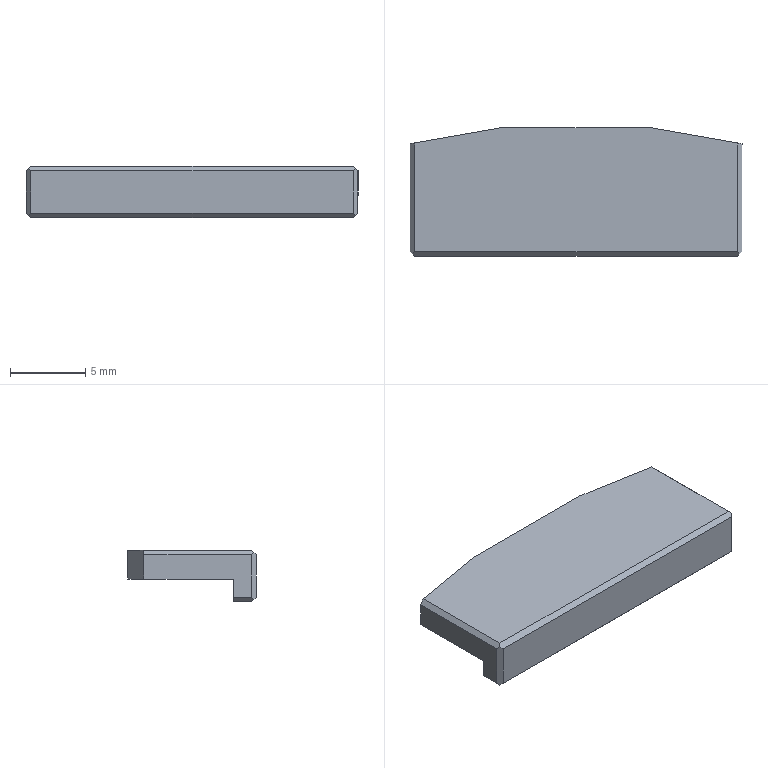Part | NX | 1 solid | 18 faces | box 22 x 8.5 x 3.4 mm | volume 389.728 mm3 | plane 18
STEP:
#1=CARTESIAN_POINT('',(-35.11,-62.629,7.853));
#2=VERTEX_POINT('',#1);
#3=CARTESIAN_POINT('',(-13.11,-62.629,7.853));
#4=VERTEX_POINT('',#3);
#5=CARTESIAN_POINT('',(-22.513,-62.629,7.853));
#6=DIRECTION('',(1.,0.,0.));
#7=VECTOR('',#6,1000.);
#8=LINE('',#5,#7);
#9=EDGE_CURVE('',#2,#4,#8,.T.);
#10=ORIENTED_EDGE('',*,*,#9,.F.);
#11=CARTESIAN_POINT('',(-35.11,-56.687,7.853));
#12=VERTEX_POINT('',#11);
#13=CARTESIAN_POINT('',(-35.11,-63.129,7.853));
#14=DIRECTION('',(0.,1.,0.));
#15=VECTOR('',#14,1000.);
#16=LINE('',#13,#15);
#17=EDGE_CURVE('',#2,#12,#16,.T.);
#18=ORIENTED_EDGE('',*,*,#17,.T.);
#19=CARTESIAN_POINT('',(-29.11,-55.629,7.853));
#20=VERTEX_POINT('',#19);
#21=CARTESIAN_POINT('',(-22.513,-54.466,7.853));
#22=DIRECTION('',(0.9848,0.1736,0.));
#23=VECTOR('',#22,1000.);
#24=LINE('',#21,#23);
#25=EDGE_CURVE('',#12,#20,#24,.T.);
#26=ORIENTED_EDGE('',*,*,#25,.T.);
#27=CARTESIAN_POINT('',(-19.11,-55.629,7.853));
#28=VERTEX_POINT('',#27);
#29=CARTESIAN_POINT('',(-22.513,-55.629,7.853));
#30=DIRECTION('',(-1.,0.,0.));
#31=VECTOR('',#30,1000.);
#32=LINE('',#29,#31);
#33=EDGE_CURVE('',#28,#20,#32,.T.);
#34=ORIENTED_EDGE('',*,*,#33,.F.);
#35=CARTESIAN_POINT('',(-13.11,-56.687,7.853));
#36=VERTEX_POINT('',#35);
#37=CARTESIAN_POINT('',(-22.513,-55.029,7.853));
#38=DIRECTION('',(0.9848,-0.1736,0.));
#39=VECTOR('',#38,1000.);
#40=LINE('',#37,#39);
#41=EDGE_CURVE('',#28,#36,#40,.T.);
#42=ORIENTED_EDGE('',*,*,#41,.T.);
#43=CARTESIAN_POINT('',(-13.11,-63.129,7.853));
#44=DIRECTION('',(0.,-1.,0.));
#45=VECTOR('',#44,1000.);
#46=LINE('',#43,#45);
#47=EDGE_CURVE('',#36,#4,#46,.T.);
#48=ORIENTED_EDGE('',*,*,#47,.T.);
#49=EDGE_LOOP('',(#10,#18,#26,#34,#42,#48));
#50=FACE_BOUND('',#49,.T.);
#51=CARTESIAN_POINT('',(-32.11,-63.129,7.853));
#52=DIRECTION('',(0.,0.,-1.));
#53=DIRECTION('',(0.,-1.,0.));
#54=AXIS2_PLACEMENT_3D('',#51,#52,#53);
#55=PLANE('',#54);
#56=ADVANCED_FACE('',(#50),#55,.T.);
#57=CARTESIAN_POINT('',(-35.11,-63.829,6.653));
#58=VERTEX_POINT('',#57);
#59=CARTESIAN_POINT('',(-35.11,-63.829,9.453));
#60=VERTEX_POINT('',#59);
#61=CARTESIAN_POINT('',(-35.11,-63.829,8.053));
#62=DIRECTION('',(0.,0.,1.));
#63=VECTOR('',#62,1000.);
#64=LINE('',#61,#63);
#65=EDGE_CURVE('',#58,#60,#64,.T.);
#66=ORIENTED_EDGE('',*,*,#65,.T.);
#67=CARTESIAN_POINT('',(-35.11,-56.687,9.453));
#68=VERTEX_POINT('',#67);
#69=CARTESIAN_POINT('',(-35.11,-60.408,9.453));
#70=DIRECTION('',(0.,1.,0.));
#71=VECTOR('',#70,1000.);
#72=LINE('',#69,#71);
#73=EDGE_CURVE('',#60,#68,#72,.T.);
#74=ORIENTED_EDGE('',*,*,#73,.T.);
#75=CARTESIAN_POINT('',(-35.11,-56.687,8.803));
#76=DIRECTION('',(0.,0.,-1.));
#77=VECTOR('',#76,1000.);
#78=LINE('',#75,#77);
#79=EDGE_CURVE('',#68,#12,#78,.T.);
#80=ORIENTED_EDGE('',*,*,#79,.T.);
#81=ORIENTED_EDGE('',*,*,#17,.F.);
#82=CARTESIAN_POINT('',(-35.11,-62.629,6.653));
#83=VERTEX_POINT('',#82);
#84=CARTESIAN_POINT('',(-35.11,-62.629,13.966));
#85=DIRECTION('',(0.,0.,1.));
#86=VECTOR('',#85,1000.);
#87=LINE('',#84,#86);
#88=EDGE_CURVE('',#83,#2,#87,.T.);
#89=ORIENTED_EDGE('',*,*,#88,.F.);
#90=CARTESIAN_POINT('',(-35.11,-63.379,6.653));
#91=DIRECTION('',(0.,1.,0.));
#92=VECTOR('',#91,1000.);
#93=LINE('',#90,#92);
#94=EDGE_CURVE('',#58,#83,#93,.T.);
#95=ORIENTED_EDGE('',*,*,#94,.F.);
#96=EDGE_LOOP('',(#66,#74,#80,#81,#89,#95));
#97=FACE_BOUND('',#96,.T.);
#98=CARTESIAN_POINT('',(-35.11,-63.129,9.253));
#99=DIRECTION('',(-1.,0.,0.));
#100=DIRECTION('',(0.,0.,1.));
#101=AXIS2_PLACEMENT_3D('',#98,#99,#100);
#102=PLANE('',#101);
#103=ADVANCED_FACE('',(#97),#102,.T.);
#104=CARTESIAN_POINT('',(-13.41,-56.634,9.753));
#105=VERTEX_POINT('',#104);
#106=CARTESIAN_POINT('',(-13.41,-63.829,9.753));
#107=VERTEX_POINT('',#106);
#108=CARTESIAN_POINT('',(-13.41,-60.408,9.753));
#109=DIRECTION('',(0.,-1.,0.));
#110=VECTOR('',#109,1000.);
#111=LINE('',#108,#110);
#112=EDGE_CURVE('',#105,#107,#111,.T.);
#113=ORIENTED_EDGE('',*,*,#112,.F.);
#114=CARTESIAN_POINT('',(-19.11,-55.629,9.753));
#115=VERTEX_POINT('',#114);
#116=CARTESIAN_POINT('',(-22.513,-55.029,9.753));
#117=DIRECTION('',(-0.9848,0.1736,0.));
#118=VECTOR('',#117,1000.);
#119=LINE('',#116,#118);
#120=EDGE_CURVE('',#105,#115,#119,.T.);
#121=ORIENTED_EDGE('',*,*,#120,.T.);
#122=CARTESIAN_POINT('',(-29.11,-55.629,9.753));
#123=VERTEX_POINT('',#122);
#124=CARTESIAN_POINT('',(-22.513,-55.629,9.753));
#125=DIRECTION('',(1.,0.,0.));
#126=VECTOR('',#125,1000.);
#127=LINE('',#124,#126);
#128=EDGE_CURVE('',#123,#115,#127,.T.);
#129=ORIENTED_EDGE('',*,*,#128,.F.);
#130=CARTESIAN_POINT('',(-34.81,-56.634,9.753));
#131=VERTEX_POINT('',#130);
#132=CARTESIAN_POINT('',(-22.513,-54.466,9.753));
#133=DIRECTION('',(-0.9848,-0.1736,0.));
#134=VECTOR('',#133,1000.);
#135=LINE('',#132,#134);
#136=EDGE_CURVE('',#123,#131,#135,.T.);
#137=ORIENTED_EDGE('',*,*,#136,.T.);
#138=CARTESIAN_POINT('',(-34.81,-63.829,9.753));
#139=VERTEX_POINT('',#138);
#140=CARTESIAN_POINT('',(-34.81,-60.408,9.753));
#141=DIRECTION('',(0.,1.,0.));
#142=VECTOR('',#141,1000.);
#143=LINE('',#140,#142);
#144=EDGE_CURVE('',#139,#131,#143,.T.);
#145=ORIENTED_EDGE('',*,*,#144,.F.);
#146=CARTESIAN_POINT('',(-24.11,-63.829,9.753));
#147=DIRECTION('',(-1.,0.,0.));
#148=VECTOR('',#147,1000.);
#149=LINE('',#146,#148);
#150=EDGE_CURVE('',#107,#139,#149,.T.);
#151=ORIENTED_EDGE('',*,*,#150,.F.);
#152=EDGE_LOOP('',(#113,#121,#129,#137,#145,#151));
#153=FACE_BOUND('',#152,.T.);
#154=CARTESIAN_POINT('',(-16.11,-63.129,9.753));
#155=DIRECTION('',(0.,0.,1.));
#156=DIRECTION('',(1.,0.,0.));
#157=AXIS2_PLACEMENT_3D('',#154,#155,#156);
#158=PLANE('',#157);
#159=ADVANCED_FACE('',(#153),#158,.T.);
#160=CARTESIAN_POINT('',(-13.11,-63.829,9.453));
#161=VERTEX_POINT('',#160);
#162=CARTESIAN_POINT('',(-13.11,-63.829,6.653));
#163=VERTEX_POINT('',#162);
#164=CARTESIAN_POINT('',(-13.11,-63.829,8.053));
#165=DIRECTION('',(0.,0.,-1.));
#166=VECTOR('',#165,1000.);
#167=LINE('',#164,#166);
#168=EDGE_CURVE('',#161,#163,#167,.T.);
#169=ORIENTED_EDGE('',*,*,#168,.T.);
#170=CARTESIAN_POINT('',(-13.11,-62.629,6.653));
#171=VERTEX_POINT('',#170);
#172=CARTESIAN_POINT('',(-13.11,-63.379,6.653));
#173=DIRECTION('',(0.,-1.,0.));
#174=VECTOR('',#173,1000.);
#175=LINE('',#172,#174);
#176=EDGE_CURVE('',#171,#163,#175,.T.);
#177=ORIENTED_EDGE('',*,*,#176,.F.);
#178=CARTESIAN_POINT('',(-13.11,-62.629,13.966));
#179=DIRECTION('',(0.,0.,-1.));
#180=VECTOR('',#179,1000.);
#181=LINE('',#178,#180);
#182=EDGE_CURVE('',#4,#171,#181,.T.);
#183=ORIENTED_EDGE('',*,*,#182,.F.);
#184=ORIENTED_EDGE('',*,*,#47,.F.);
#185=CARTESIAN_POINT('',(-13.11,-56.687,9.453));
#186=VERTEX_POINT('',#185);
#187=CARTESIAN_POINT('',(-13.11,-56.687,8.803));
#188=DIRECTION('',(0.,0.,1.));
#189=VECTOR('',#188,1000.);
#190=LINE('',#187,#189);
#191=EDGE_CURVE('',#36,#186,#190,.T.);
#192=ORIENTED_EDGE('',*,*,#191,.T.);
#193=CARTESIAN_POINT('',(-13.11,-60.408,9.453));
#194=DIRECTION('',(0.,-1.,0.));
#195=VECTOR('',#194,1000.);
#196=LINE('',#193,#195);
#197=EDGE_CURVE('',#186,#161,#196,.T.);
#198=ORIENTED_EDGE('',*,*,#197,.T.);
#199=EDGE_LOOP('',(#169,#177,#183,#184,#192,#198));
#200=FACE_BOUND('',#199,.T.);
#201=CARTESIAN_POINT('',(-13.11,-63.129,7.853));
#202=DIRECTION('',(1.,0.,0.));
#203=DIRECTION('',(0.,-1.,0.));
#204=AXIS2_PLACEMENT_3D('',#201,#202,#203);
#205=PLANE('',#204);
#206=ADVANCED_FACE('',(#200),#205,.T.);
#207=CARTESIAN_POINT('',(-34.81,-63.829,6.353));
#208=VERTEX_POINT('',#207);
#209=CARTESIAN_POINT('',(-34.81,-62.629,6.353));
#210=VERTEX_POINT('',#209);
#211=CARTESIAN_POINT('',(-34.81,-63.379,6.353));
#212=DIRECTION('',(0.,1.,0.));
#213=VECTOR('',#212,1000.);
#214=LINE('',#211,#213);
#215=EDGE_CURVE('',#208,#210,#214,.T.);
#216=ORIENTED_EDGE('',*,*,#215,.T.);
#217=CARTESIAN_POINT('',(-13.41,-62.629,6.353));
#218=VERTEX_POINT('',#217);
#219=CARTESIAN_POINT('',(-22.513,-62.629,6.353));
#220=DIRECTION('',(1.,0.,0.));
#221=VECTOR('',#220,1000.);
#222=LINE('',#219,#221);
#223=EDGE_CURVE('',#210,#218,#222,.T.);
#224=ORIENTED_EDGE('',*,*,#223,.T.);
#225=CARTESIAN_POINT('',(-13.41,-63.829,6.353));
#226=VERTEX_POINT('',#225);
#227=CARTESIAN_POINT('',(-13.41,-63.379,6.353));
#228=DIRECTION('',(0.,-1.,0.));
#229=VECTOR('',#228,1000.);
#230=LINE('',#227,#229);
#231=EDGE_CURVE('',#218,#226,#230,.T.);
#232=ORIENTED_EDGE('',*,*,#231,.T.);
#233=CARTESIAN_POINT('',(-24.11,-63.829,6.353));
#234=DIRECTION('',(-1.,0.,0.));
#235=VECTOR('',#234,1000.);
#236=LINE('',#233,#235);
#237=EDGE_CURVE('',#226,#208,#236,.T.);
#238=ORIENTED_EDGE('',*,*,#237,.T.);
#239=EDGE_LOOP('',(#216,#224,#232,#238));
#240=FACE_BOUND('',#239,.T.);
#241=CARTESIAN_POINT('',(-19.282,-63.809,6.353));
#242=DIRECTION('',(0.,0.,-1.));
#243=DIRECTION('',(0.,-1.,0.));
#244=AXIS2_PLACEMENT_3D('',#241,#242,#243);
#245=PLANE('',#244);
#246=ADVANCED_FACE('',(#240),#245,.T.);
#247=ORIENTED_EDGE('',*,*,#73,.F.);
#248=CARTESIAN_POINT('',(-34.96,-63.979,9.603));
#249=VERTEX_POINT('',#248);
#250=CARTESIAN_POINT('',(-22.513,-76.426,22.05));
#251=DIRECTION('',(0.5774,-0.5774,0.5774));
#252=VECTOR('',#251,1000.);
#253=LINE('',#250,#252);
#254=EDGE_CURVE('',#60,#249,#253,.T.);
#255=ORIENTED_EDGE('',*,*,#254,.T.);
#256=CARTESIAN_POINT('',(-22.513,-51.532,22.05));
#257=DIRECTION('',(0.5774,0.5774,0.5774));
#258=VECTOR('',#257,1000.);
#259=LINE('',#256,#258);
#260=EDGE_CURVE('',#249,#139,#259,.T.);
#261=ORIENTED_EDGE('',*,*,#260,.T.);
#262=ORIENTED_EDGE('',*,*,#144,.T.);
#263=CARTESIAN_POINT('',(-22.513,-54.466,22.05));
#264=DIRECTION('',(0.7017,0.1237,0.7017));
#265=VECTOR('',#264,1000.);
#266=LINE('',#263,#265);
#267=EDGE_CURVE('',#68,#131,#266,.T.);
#268=ORIENTED_EDGE('',*,*,#267,.F.);
#269=EDGE_LOOP('',(#247,#255,#261,#262,#268));
#270=FACE_BOUND('',#269,.T.);
#271=CARTESIAN_POINT('',(-34.96,-60.408,9.603));
#272=DIRECTION('',(-0.7071,0.,0.7071));
#273=DIRECTION('',(0.,1.,0.));
#274=AXIS2_PLACEMENT_3D('',#271,#272,#273);
#275=PLANE('',#274);
#276=ADVANCED_FACE('',(#270),#275,.T.);
#277=ORIENTED_EDGE('',*,*,#237,.F.);
#278=CARTESIAN_POINT('',(-13.26,-63.979,6.503));
#279=VERTEX_POINT('',#278);
#280=CARTESIAN_POINT('',(-22.513,-54.726,-2.75));
#281=DIRECTION('',(0.5774,-0.5774,0.5774));
#282=VECTOR('',#281,1000.);
#283=LINE('',#280,#282);
#284=EDGE_CURVE('',#226,#279,#283,.T.);
#285=ORIENTED_EDGE('',*,*,#284,.T.);
#286=CARTESIAN_POINT('',(-13.41,-64.129,6.653));
#287=VERTEX_POINT('',#286);
#288=CARTESIAN_POINT('',(-22.513,-73.232,15.756));
#289=DIRECTION('',(0.5774,0.5774,-0.5774));
#290=VECTOR('',#289,1000.);
#291=LINE('',#288,#290);
#292=EDGE_CURVE('',#287,#279,#291,.T.);
#293=ORIENTED_EDGE('',*,*,#292,.F.);
#294=CARTESIAN_POINT('',(-34.81,-64.129,6.653));
#295=VERTEX_POINT('',#294);
#296=CARTESIAN_POINT('',(-24.11,-64.129,6.653));
#297=DIRECTION('',(-1.,0.,0.));
#298=VECTOR('',#297,1000.);
#299=LINE('',#296,#298);
#300=EDGE_CURVE('',#287,#295,#299,.T.);
#301=ORIENTED_EDGE('',*,*,#300,.T.);
#302=CARTESIAN_POINT('',(-34.96,-63.979,6.503));
#303=VERTEX_POINT('',#302);
#304=CARTESIAN_POINT('',(-22.513,-76.426,18.95));
#305=DIRECTION('',(-0.5774,0.5774,-0.5774));
#306=VECTOR('',#305,1000.);
#307=LINE('',#304,#306);
#308=EDGE_CURVE('',#295,#303,#307,.T.);
#309=ORIENTED_EDGE('',*,*,#308,.T.);
#310=CARTESIAN_POINT('',(-22.513,-51.532,-5.944));
#311=DIRECTION('',(0.5774,0.5774,-0.5774));
#312=VECTOR('',#311,1000.);
#313=LINE('',#310,#312);
#314=EDGE_CURVE('',#303,#208,#313,.T.);
#315=ORIENTED_EDGE('',*,*,#314,.T.);
#316=EDGE_LOOP('',(#277,#285,#293,#301,#309,#315));
#317=FACE_BOUND('',#316,.T.);
#318=CARTESIAN_POINT('',(-24.11,-63.979,6.503));
#319=DIRECTION('',(0.,-0.7071,-0.7071));
#320=DIRECTION('',(0.,-0.7071,0.7071));
#321=AXIS2_PLACEMENT_3D('',#318,#319,#320);
#322=PLANE('',#321);
#323=ADVANCED_FACE('',(#317),#322,.T.);
#324=ORIENTED_EDGE('',*,*,#65,.F.);
#325=CARTESIAN_POINT('',(-22.513,-76.426,-5.944));
#326=DIRECTION('',(0.5774,-0.5774,-0.5774));
#327=VECTOR('',#326,1000.);
#328=LINE('',#325,#327);
#329=EDGE_CURVE('',#58,#303,#328,.T.);
#330=ORIENTED_EDGE('',*,*,#329,.T.);
#331=ORIENTED_EDGE('',*,*,#308,.F.);
#332=CARTESIAN_POINT('',(-34.81,-64.129,9.453));
#333=VERTEX_POINT('',#332);
#334=CARTESIAN_POINT('',(-34.81,-64.129,8.053));
#335=DIRECTION('',(0.,0.,1.));
#336=VECTOR('',#335,1000.);
#337=LINE('',#334,#336);
#338=EDGE_CURVE('',#295,#333,#337,.T.);
#339=ORIENTED_EDGE('',*,*,#338,.T.);
#340=CARTESIAN_POINT('',(-22.513,-76.426,-2.844));
#341=DIRECTION('',(0.5774,-0.5774,-0.5774));
#342=VECTOR('',#341,1000.);
#343=LINE('',#340,#342);
#344=EDGE_CURVE('',#249,#333,#343,.T.);
#345=ORIENTED_EDGE('',*,*,#344,.F.);
#346=ORIENTED_EDGE('',*,*,#254,.F.);
#347=EDGE_LOOP('',(#324,#330,#331,#339,#345,#346));
#348=FACE_BOUND('',#347,.T.);
#349=CARTESIAN_POINT('',(-34.96,-63.979,8.053));
#350=DIRECTION('',(-0.7071,-0.7071,0.));
#351=DIRECTION('',(-0.7071,0.7071,0.));
#352=AXIS2_PLACEMENT_3D('',#349,#350,#351);
#353=PLANE('',#352);
#354=ADVANCED_FACE('',(#348),#353,.T.);
#355=ORIENTED_EDGE('',*,*,#112,.T.);
#356=CARTESIAN_POINT('',(-13.26,-63.979,9.603));
#357=VERTEX_POINT('',#356);
#358=CARTESIAN_POINT('',(-22.513,-54.726,18.856));
#359=DIRECTION('',(0.5774,-0.5774,-0.5774));
#360=VECTOR('',#359,1000.);
#361=LINE('',#358,#360);
#362=EDGE_CURVE('',#107,#357,#361,.T.);
#363=ORIENTED_EDGE('',*,*,#362,.T.);
#364=CARTESIAN_POINT('',(-22.513,-73.232,18.856));
#365=DIRECTION('',(0.5774,0.5774,-0.5774));
#366=VECTOR('',#365,1000.);
#367=LINE('',#364,#366);
#368=EDGE_CURVE('',#357,#161,#367,.T.);
#369=ORIENTED_EDGE('',*,*,#368,.T.);
#370=ORIENTED_EDGE('',*,*,#197,.F.);
#371=CARTESIAN_POINT('',(-22.513,-55.029,18.856));
#372=DIRECTION('',(-0.7017,0.1237,0.7017));
#373=VECTOR('',#372,1000.);
#374=LINE('',#371,#373);
#375=EDGE_CURVE('',#186,#105,#374,.T.);
#376=ORIENTED_EDGE('',*,*,#375,.T.);
#377=EDGE_LOOP('',(#355,#363,#369,#370,#376));
#378=FACE_BOUND('',#377,.T.);
#379=CARTESIAN_POINT('',(-13.26,-60.408,9.603));
#380=DIRECTION('',(-0.7071,0.,-0.7071));
#381=DIRECTION('',(-0.7071,0.,0.7071));
#382=AXIS2_PLACEMENT_3D('',#379,#380,#381);
#383=PLANE('',#382);
#384=ADVANCED_FACE('',(#378),#383,.F.);
#385=ORIENTED_EDGE('',*,*,#231,.F.);
#386=CARTESIAN_POINT('',(-22.513,-62.629,-2.75));
#387=DIRECTION('',(0.7071,0.,0.7071));
#388=VECTOR('',#387,1000.);
#389=LINE('',#386,#388);
#390=EDGE_CURVE('',#218,#171,#389,.T.);
#391=ORIENTED_EDGE('',*,*,#390,.T.);
#392=ORIENTED_EDGE('',*,*,#176,.T.);
#393=CARTESIAN_POINT('',(-22.513,-73.232,-2.75));
#394=DIRECTION('',(-0.5774,-0.5774,-0.5774));
#395=VECTOR('',#394,1000.);
#396=LINE('',#393,#395);
#397=EDGE_CURVE('',#163,#279,#396,.T.);
#398=ORIENTED_EDGE('',*,*,#397,.T.);
#399=ORIENTED_EDGE('',*,*,#284,.F.);
#400=EDGE_LOOP('',(#385,#391,#392,#398,#399));
#401=FACE_BOUND('',#400,.T.);
#402=CARTESIAN_POINT('',(-13.26,-63.379,6.503));
#403=DIRECTION('',(0.7071,0.,-0.7071));
#404=DIRECTION('',(0.,-1.,0.));
#405=AXIS2_PLACEMENT_3D('',#402,#403,#404);
#406=PLANE('',#405);
#407=ADVANCED_FACE('',(#401),#406,.T.);
#408=ORIENTED_EDGE('',*,*,#215,.F.);
#409=ORIENTED_EDGE('',*,*,#314,.F.);
#410=ORIENTED_EDGE('',*,*,#329,.F.);
#411=ORIENTED_EDGE('',*,*,#94,.T.);
#412=CARTESIAN_POINT('',(-22.513,-62.629,-5.944));
#413=DIRECTION('',(0.7071,0.,-0.7071));
#414=VECTOR('',#413,1000.);
#415=LINE('',#412,#414);
#416=EDGE_CURVE('',#83,#210,#415,.T.);
#417=ORIENTED_EDGE('',*,*,#416,.T.);
#418=EDGE_LOOP('',(#408,#409,#410,#411,#417));
#419=FACE_BOUND('',#418,.T.);
#420=CARTESIAN_POINT('',(-34.96,-63.379,6.503));
#421=DIRECTION('',(-0.7071,0.,-0.7071));
#422=DIRECTION('',(-0.7071,0.,0.7071));
#423=AXIS2_PLACEMENT_3D('',#420,#421,#422);
#424=PLANE('',#423);
#425=ADVANCED_FACE('',(#419),#424,.T.);
#426=CARTESIAN_POINT('',(-29.11,-55.629,8.803));
#427=DIRECTION('',(0.,0.,-1.));
#428=VECTOR('',#427,1000.);
#429=LINE('',#426,#428);
#430=EDGE_CURVE('',#123,#20,#429,.T.);
#431=ORIENTED_EDGE('',*,*,#430,.F.);
#432=ORIENTED_EDGE('',*,*,#128,.T.);
#433=CARTESIAN_POINT('',(-19.11,-55.629,8.803));
#434=DIRECTION('',(0.,0.,1.));
#435=VECTOR('',#434,1000.);
#436=LINE('',#433,#435);
#437=EDGE_CURVE('',#28,#115,#436,.T.);
#438=ORIENTED_EDGE('',*,*,#437,.F.);
#439=ORIENTED_EDGE('',*,*,#33,.T.);
#440=EDGE_LOOP('',(#431,#432,#438,#439));
#441=FACE_BOUND('',#440,.T.);
#442=CARTESIAN_POINT('',(-22.513,-55.629,13.966));
#443=DIRECTION('',(0.,-1.,0.));
#444=DIRECTION('',(-1.,0.,0.));
#445=AXIS2_PLACEMENT_3D('',#442,#443,#444);
#446=PLANE('',#445);
#447=ADVANCED_FACE('',(#441),#446,.F.);
#448=ORIENTED_EDGE('',*,*,#437,.T.);
#449=ORIENTED_EDGE('',*,*,#120,.F.);
#450=ORIENTED_EDGE('',*,*,#375,.F.);
#451=ORIENTED_EDGE('',*,*,#191,.F.);
#452=ORIENTED_EDGE('',*,*,#41,.F.);
#453=EDGE_LOOP('',(#448,#449,#450,#451,#452));
#454=FACE_BOUND('',#453,.T.);
#455=CARTESIAN_POINT('',(-16.11,-56.158,8.803));
#456=DIRECTION('',(-0.1736,-0.9848,0.));
#457=DIRECTION('',(-0.9848,0.1736,0.));
#458=AXIS2_PLACEMENT_3D('',#455,#456,#457);
#459=PLANE('',#458);
#460=ADVANCED_FACE('',(#454),#459,.F.);
#461=ORIENTED_EDGE('',*,*,#430,.T.);
#462=ORIENTED_EDGE('',*,*,#25,.F.);
#463=ORIENTED_EDGE('',*,*,#79,.F.);
#464=ORIENTED_EDGE('',*,*,#267,.T.);
#465=ORIENTED_EDGE('',*,*,#136,.F.);
#466=EDGE_LOOP('',(#461,#462,#463,#464,#465));
#467=FACE_BOUND('',#466,.T.);
#468=CARTESIAN_POINT('',(-32.11,-56.158,8.803));
#469=DIRECTION('',(0.1736,-0.9848,0.));
#470=DIRECTION('',(0.,0.,-1.));
#471=AXIS2_PLACEMENT_3D('',#468,#469,#470);
#472=PLANE('',#471);
#473=ADVANCED_FACE('',(#467),#472,.F.);
#474=CARTESIAN_POINT('',(-13.41,-64.129,9.453));
#475=VERTEX_POINT('',#474);
#476=CARTESIAN_POINT('',(-13.41,-64.129,8.053));
#477=DIRECTION('',(0.,0.,-1.));
#478=VECTOR('',#477,1000.);
#479=LINE('',#476,#478);
#480=EDGE_CURVE('',#475,#287,#479,.T.);
#481=ORIENTED_EDGE('',*,*,#480,.F.);
#482=CARTESIAN_POINT('',(-24.11,-64.129,9.453));
#483=DIRECTION('',(-1.,0.,0.));
#484=VECTOR('',#483,1000.);
#485=LINE('',#482,#484);
#486=EDGE_CURVE('',#475,#333,#485,.T.);
#487=ORIENTED_EDGE('',*,*,#486,.T.);
#488=ORIENTED_EDGE('',*,*,#338,.F.);
#489=ORIENTED_EDGE('',*,*,#300,.F.);
#490=EDGE_LOOP('',(#481,#487,#488,#489));
#491=FACE_BOUND('',#490,.T.);
#492=CARTESIAN_POINT('',(-22.513,-64.129,13.966));
#493=DIRECTION('',(0.,-1.,0.));
#494=DIRECTION('',(-1.,0.,0.));
#495=AXIS2_PLACEMENT_3D('',#492,#493,#494);
#496=PLANE('',#495);
#497=ADVANCED_FACE('',(#491),#496,.T.);
#498=ORIENTED_EDGE('',*,*,#9,.T.);
#499=ORIENTED_EDGE('',*,*,#182,.T.);
#500=ORIENTED_EDGE('',*,*,#390,.F.);
#501=ORIENTED_EDGE('',*,*,#223,.F.);
#502=ORIENTED_EDGE('',*,*,#416,.F.);
#503=ORIENTED_EDGE('',*,*,#88,.T.);
#504=EDGE_LOOP('',(#498,#499,#500,#501,#502,#503));
#505=FACE_BOUND('',#504,.T.);
#506=CARTESIAN_POINT('',(-16.21,-62.629,7.853));
#507=DIRECTION('',(0.,1.,0.));
#508=DIRECTION('',(1.,0.,0.));
#509=AXIS2_PLACEMENT_3D('',#506,#507,#508);
#510=PLANE('',#509);
#511=ADVANCED_FACE('',(#505),#510,.T.);
#512=ORIENTED_EDGE('',*,*,#486,.F.);
#513=CARTESIAN_POINT('',(-22.513,-73.232,0.3502));
#514=DIRECTION('',(-0.5774,-0.5774,-0.5774));
#515=VECTOR('',#514,1000.);
#516=LINE('',#513,#515);
#517=EDGE_CURVE('',#357,#475,#516,.T.);
#518=ORIENTED_EDGE('',*,*,#517,.F.);
#519=ORIENTED_EDGE('',*,*,#362,.F.);
#520=ORIENTED_EDGE('',*,*,#150,.T.);
#521=ORIENTED_EDGE('',*,*,#260,.F.);
#522=ORIENTED_EDGE('',*,*,#344,.T.);
#523=EDGE_LOOP('',(#512,#518,#519,#520,#521,#522));
#524=FACE_BOUND('',#523,.T.);
#525=CARTESIAN_POINT('',(-24.11,-63.979,9.603));
#526=DIRECTION('',(0.,-0.7071,0.7071));
#527=DIRECTION('',(-1.,0.,0.));
#528=AXIS2_PLACEMENT_3D('',#525,#526,#527);
#529=PLANE('',#528);
#530=ADVANCED_FACE('',(#524),#529,.T.);
#531=ORIENTED_EDGE('',*,*,#480,.T.);
#532=ORIENTED_EDGE('',*,*,#292,.T.);
#533=ORIENTED_EDGE('',*,*,#397,.F.);
#534=ORIENTED_EDGE('',*,*,#168,.F.);
#535=ORIENTED_EDGE('',*,*,#368,.F.);
#536=ORIENTED_EDGE('',*,*,#517,.T.);
#537=EDGE_LOOP('',(#531,#532,#533,#534,#535,#536));
#538=FACE_BOUND('',#537,.T.);
#539=CARTESIAN_POINT('',(-13.26,-63.979,8.053));
#540=DIRECTION('',(-0.7071,0.7071,0.));
#541=DIRECTION('',(0.,0.,1.));
#542=AXIS2_PLACEMENT_3D('',#539,#540,#541);
#543=PLANE('',#542);
#544=ADVANCED_FACE('',(#538),#543,.F.);
#545=CLOSED_SHELL('',(#56,#103,#159,#206,#246,#276,#323,#354,#384,#407,#425,#447,#460,#473,#497,#511,#530,#544));
#546=MANIFOLD_SOLID_BREP('',#545);
#547=(LENGTH_UNIT()NAMED_UNIT(*)SI_UNIT(.MILLI.,.METRE.));
#548=UNCERTAINTY_MEASURE_WITH_UNIT(LENGTH_MEASURE(0.00001),#547,'','');
#549=(NAMED_UNIT(*)PLANE_ANGLE_UNIT()SI_UNIT($,.RADIAN.));
#550=(NAMED_UNIT(*)SI_UNIT($,.STERADIAN.)SOLID_ANGLE_UNIT());
#551=(GEOMETRIC_REPRESENTATION_CONTEXT(3)GLOBAL_UNCERTAINTY_ASSIGNED_CONTEXT((#548))GLOBAL_UNIT_ASSIGNED_CONTEXT((#547,#549,#550))REPRESENTATION_CONTEXT('',''));
#552=ADVANCED_BREP_SHAPE_REPRESENTATION('',(#546),#551);